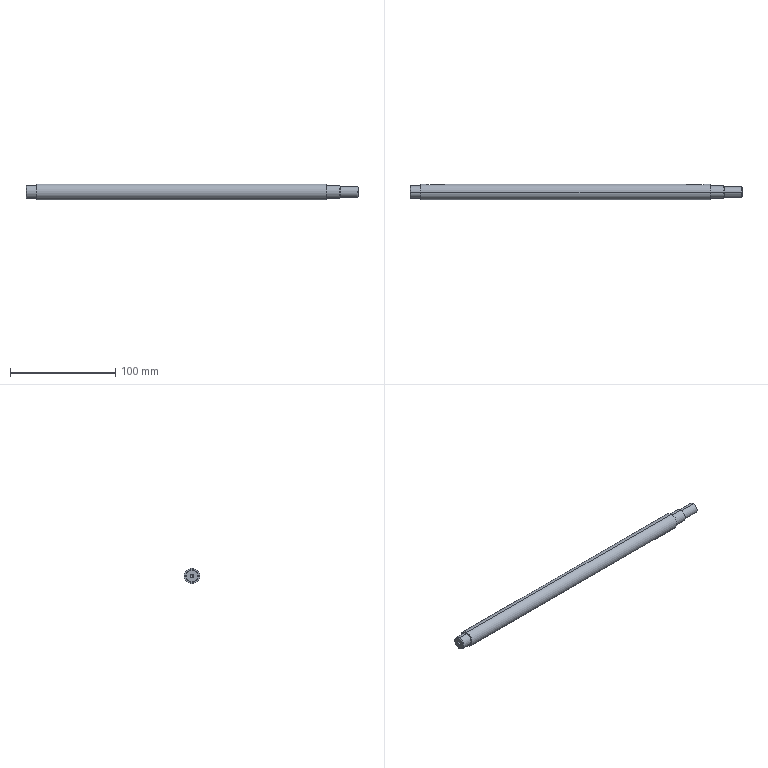Part | STEP file | 11-SS10911 | 1 solid | 42 faces | box 315 x 15 x 15 mm | volume 51716 mm3 | cylinder 18 | plane 14 | cone 10 | commonest cylinder face diameters 3.3 x4 5 x4 12 x4 3 x2 10 x2 15 x2
STEP:
#1=CARTESIAN_POINT('',(304.9,0.,1.65));
#2=VERTEX_POINT('',#1);
#3=CARTESIAN_POINT('',(304.9,0.,-1.65));
#4=VERTEX_POINT('',#3);
#5=CARTESIAN_POINT('',(304.9,0.,0.));
#6=DIRECTION('',(1.,0.,0.));
#7=DIRECTION('',(0.,0.,-1.));
#8=AXIS2_PLACEMENT_3D('',#5,#6,#7);
#9=CIRCLE('',#8,1.65);
#10=EDGE_CURVE('',#2,#4,#9,.T.);
#11=ORIENTED_EDGE('',*,*,#10,.F.);
#12=CARTESIAN_POINT('',(315.,0.,1.65));
#13=VERTEX_POINT('',#12);
#14=CARTESIAN_POINT('',(315.,0.,1.65));
#15=DIRECTION('',(1.,0.,0.));
#16=VECTOR('',#15,1000.);
#17=LINE('',#14,#16);
#18=EDGE_CURVE('',#2,#13,#17,.T.);
#19=ORIENTED_EDGE('',*,*,#18,.T.);
#20=CARTESIAN_POINT('',(315.,0.,-1.65));
#21=VERTEX_POINT('',#20);
#22=CARTESIAN_POINT('',(315.,0.,0.));
#23=DIRECTION('',(1.,0.,0.));
#24=DIRECTION('',(0.,0.,-1.));
#25=AXIS2_PLACEMENT_3D('',#22,#23,#24);
#26=CIRCLE('',#25,1.65);
#27=EDGE_CURVE('',#13,#21,#26,.T.);
#28=ORIENTED_EDGE('',*,*,#27,.T.);
#29=CARTESIAN_POINT('',(315.,0.,-1.65));
#30=DIRECTION('',(1.,0.,0.));
#31=VECTOR('',#30,1000.);
#32=LINE('',#29,#31);
#33=EDGE_CURVE('',#4,#21,#32,.T.);
#34=ORIENTED_EDGE('',*,*,#33,.F.);
#35=EDGE_LOOP('',(#11,#19,#28,#34));
#36=FACE_OUTER_BOUND('',#35,.T.);
#37=CARTESIAN_POINT('',(315.,0.,0.));
#38=DIRECTION('',(1.,0.,0.));
#39=DIRECTION('',(0.,0.,-1.));
#40=AXIS2_PLACEMENT_3D('',#37,#38,#39);
#41=CYLINDRICAL_SURFACE('',#40,1.65);
#42=ADVANCED_FACE('',(#36),#41,.F.);
#43=CARTESIAN_POINT('',(303.909,0.,0.));
#44=VERTEX_POINT('',#43);
#45=CARTESIAN_POINT('',(304.9,0.,-1.65));
#46=DIRECTION('',(0.515,0.,-0.8572));
#47=VECTOR('',#46,1000.);
#48=LINE('',#45,#47);
#49=EDGE_CURVE('',#44,#4,#48,.T.);
#50=ORIENTED_EDGE('',*,*,#49,.F.);
#51=CARTESIAN_POINT('',(304.9,0.,1.65));
#52=DIRECTION('',(0.515,0.,0.8572));
#53=VECTOR('',#52,1000.);
#54=LINE('',#51,#53);
#55=EDGE_CURVE('',#44,#2,#54,.T.);
#56=ORIENTED_EDGE('',*,*,#55,.T.);
#57=ORIENTED_EDGE('',*,*,#10,.T.);
#58=EDGE_LOOP('',(#50,#56,#57));
#59=FACE_OUTER_BOUND('',#58,.T.);
#60=CARTESIAN_POINT('',(304.9,0.,0.));
#61=DIRECTION('',(1.,0.,0.));
#62=DIRECTION('',(0.,0.,-1.));
#63=AXIS2_PLACEMENT_3D('',#60,#61,#62);
#64=CONICAL_SURFACE('',#63,1.65,1.03);
#65=ADVANCED_FACE('',(#59),#64,.F.);
#66=CARTESIAN_POINT('',(10.1,0.,-1.65));
#67=VERTEX_POINT('',#66);
#68=CARTESIAN_POINT('',(10.1,0.,1.65));
#69=VERTEX_POINT('',#68);
#70=CARTESIAN_POINT('',(10.1,0.,0.));
#71=DIRECTION('',(-1.,0.,0.));
#72=DIRECTION('',(0.,0.,1.));
#73=AXIS2_PLACEMENT_3D('',#70,#71,#72);
#74=CIRCLE('',#73,1.65);
#75=EDGE_CURVE('',#67,#69,#74,.T.);
#76=ORIENTED_EDGE('',*,*,#75,.F.);
#77=CARTESIAN_POINT('',(0.,0.,-1.65));
#78=VERTEX_POINT('',#77);
#79=CARTESIAN_POINT('',(0.,0.,-1.65));
#80=DIRECTION('',(-1.,0.,0.));
#81=VECTOR('',#80,1000.);
#82=LINE('',#79,#81);
#83=EDGE_CURVE('',#67,#78,#82,.T.);
#84=ORIENTED_EDGE('',*,*,#83,.T.);
#85=CARTESIAN_POINT('',(0.,0.,1.65));
#86=VERTEX_POINT('',#85);
#87=CARTESIAN_POINT('',(0.,0.,0.));
#88=DIRECTION('',(-1.,0.,0.));
#89=DIRECTION('',(0.,0.,1.));
#90=AXIS2_PLACEMENT_3D('',#87,#88,#89);
#91=CIRCLE('',#90,1.65);
#92=EDGE_CURVE('',#78,#86,#91,.T.);
#93=ORIENTED_EDGE('',*,*,#92,.T.);
#94=CARTESIAN_POINT('',(0.,0.,1.65));
#95=DIRECTION('',(-1.,0.,0.));
#96=VECTOR('',#95,1000.);
#97=LINE('',#94,#96);
#98=EDGE_CURVE('',#69,#86,#97,.T.);
#99=ORIENTED_EDGE('',*,*,#98,.F.);
#100=EDGE_LOOP('',(#76,#84,#93,#99));
#101=FACE_OUTER_BOUND('',#100,.T.);
#102=CARTESIAN_POINT('',(0.,0.,0.));
#103=DIRECTION('',(-1.,0.,0.));
#104=DIRECTION('',(0.,0.,1.));
#105=AXIS2_PLACEMENT_3D('',#102,#103,#104);
#106=CYLINDRICAL_SURFACE('',#105,1.65);
#107=ADVANCED_FACE('',(#101),#106,.F.);
#108=CARTESIAN_POINT('',(11.091,0.,0.));
#109=VERTEX_POINT('',#108);
#110=CARTESIAN_POINT('',(10.1,0.,1.65));
#111=DIRECTION('',(-0.515,0.,0.8572));
#112=VECTOR('',#111,1000.);
#113=LINE('',#110,#112);
#114=EDGE_CURVE('',#109,#69,#113,.T.);
#115=ORIENTED_EDGE('',*,*,#114,.F.);
#116=CARTESIAN_POINT('',(10.1,0.,-1.65));
#117=DIRECTION('',(-0.515,0.,-0.8572));
#118=VECTOR('',#117,1000.);
#119=LINE('',#116,#118);
#120=EDGE_CURVE('',#109,#67,#119,.T.);
#121=ORIENTED_EDGE('',*,*,#120,.T.);
#122=ORIENTED_EDGE('',*,*,#75,.T.);
#123=EDGE_LOOP('',(#115,#121,#122));
#124=FACE_OUTER_BOUND('',#123,.T.);
#125=CARTESIAN_POINT('',(10.1,0.,0.));
#126=DIRECTION('',(-1.,0.,0.));
#127=DIRECTION('',(0.,0.,1.));
#128=AXIS2_PLACEMENT_3D('',#125,#126,#127);
#129=CONICAL_SURFACE('',#128,1.65,1.03);
#130=ADVANCED_FACE('',(#124),#129,.F.);
#131=CARTESIAN_POINT('',(298.,0.,-5.5));
#132=VERTEX_POINT('',#131);
#133=CARTESIAN_POINT('',(298.,0.,5.5));
#134=VERTEX_POINT('',#133);
#135=CARTESIAN_POINT('',(298.,0.,0.));
#136=DIRECTION('',(1.,0.,0.));
#137=DIRECTION('',(0.,0.,1.));
#138=AXIS2_PLACEMENT_3D('',#135,#136,#137);
#139=CIRCLE('',#138,5.5);
#140=EDGE_CURVE('',#132,#134,#139,.T.);
#141=ORIENTED_EDGE('',*,*,#140,.F.);
#142=CARTESIAN_POINT('',(297.5,0.,-6.));
#143=VERTEX_POINT('',#142);
#144=CARTESIAN_POINT('',(297.5,0.,-6.));
#145=DIRECTION('',(-0.7071,0.,-0.7071));
#146=VECTOR('',#145,1000.);
#147=LINE('',#144,#146);
#148=EDGE_CURVE('',#132,#143,#147,.T.);
#149=ORIENTED_EDGE('',*,*,#148,.T.);
#150=CARTESIAN_POINT('',(297.5,0.,6.));
#151=VERTEX_POINT('',#150);
#152=CARTESIAN_POINT('',(297.5,0.,0.));
#153=DIRECTION('',(-1.,0.,0.));
#154=DIRECTION('',(0.,0.,1.));
#155=AXIS2_PLACEMENT_3D('',#152,#153,#154);
#156=CIRCLE('',#155,6.);
#157=EDGE_CURVE('',#151,#143,#156,.T.);
#158=ORIENTED_EDGE('',*,*,#157,.F.);
#159=CARTESIAN_POINT('',(297.5,0.,6.));
#160=DIRECTION('',(-0.7071,0.,0.7071));
#161=VECTOR('',#160,1000.);
#162=LINE('',#159,#161);
#163=EDGE_CURVE('',#134,#151,#162,.T.);
#164=ORIENTED_EDGE('',*,*,#163,.F.);
#165=EDGE_LOOP('',(#141,#149,#158,#164));
#166=FACE_OUTER_BOUND('',#165,.T.);
#167=CARTESIAN_POINT('',(297.5,0.,0.));
#168=DIRECTION('',(-1.,0.,0.));
#169=DIRECTION('',(0.,0.,1.));
#170=AXIS2_PLACEMENT_3D('',#167,#168,#169);
#171=CONICAL_SURFACE('',#170,6.,0.7854);
#172=ADVANCED_FACE('',(#166),#171,.T.);
#173=CARTESIAN_POINT('',(315.,0.,-4.5));
#174=VERTEX_POINT('',#173);
#175=CARTESIAN_POINT('',(315.,0.,4.5));
#176=VERTEX_POINT('',#175);
#177=CARTESIAN_POINT('',(315.,0.,0.));
#178=DIRECTION('',(1.,0.,0.));
#179=DIRECTION('',(0.,0.,1.));
#180=AXIS2_PLACEMENT_3D('',#177,#178,#179);
#181=CIRCLE('',#180,4.5);
#182=EDGE_CURVE('',#174,#176,#181,.T.);
#183=ORIENTED_EDGE('',*,*,#182,.F.);
#184=CARTESIAN_POINT('',(314.5,0.,-5.));
#185=VERTEX_POINT('',#184);
#186=CARTESIAN_POINT('',(314.5,0.,-5.));
#187=DIRECTION('',(-0.7071,0.,-0.7071));
#188=VECTOR('',#187,1000.);
#189=LINE('',#186,#188);
#190=EDGE_CURVE('',#174,#185,#189,.T.);
#191=ORIENTED_EDGE('',*,*,#190,.T.);
#192=CARTESIAN_POINT('',(314.5,0.,5.));
#193=VERTEX_POINT('',#192);
#194=CARTESIAN_POINT('',(314.5,0.,0.));
#195=DIRECTION('',(-1.,0.,0.));
#196=DIRECTION('',(0.,0.,1.));
#197=AXIS2_PLACEMENT_3D('',#194,#195,#196);
#198=CIRCLE('',#197,5.);
#199=EDGE_CURVE('',#193,#185,#198,.T.);
#200=ORIENTED_EDGE('',*,*,#199,.F.);
#201=CARTESIAN_POINT('',(314.5,0.,5.));
#202=DIRECTION('',(-0.7071,0.,0.7071));
#203=VECTOR('',#202,1000.);
#204=LINE('',#201,#203);
#205=EDGE_CURVE('',#176,#193,#204,.T.);
#206=ORIENTED_EDGE('',*,*,#205,.F.);
#207=EDGE_LOOP('',(#183,#191,#200,#206));
#208=FACE_OUTER_BOUND('',#207,.T.);
#209=CARTESIAN_POINT('',(314.5,0.,0.));
#210=DIRECTION('',(-1.,0.,0.));
#211=DIRECTION('',(0.,0.,1.));
#212=AXIS2_PLACEMENT_3D('',#209,#210,#211);
#213=CONICAL_SURFACE('',#212,5.,0.7854);
#214=ADVANCED_FACE('',(#208),#213,.T.);
#215=CARTESIAN_POINT('',(0.,0.,5.5));
#216=VERTEX_POINT('',#215);
#217=CARTESIAN_POINT('',(0.,0.,-5.5));
#218=VERTEX_POINT('',#217);
#219=CARTESIAN_POINT('',(0.,0.,0.));
#220=DIRECTION('',(-1.,0.,0.));
#221=DIRECTION('',(0.,0.,-1.));
#222=AXIS2_PLACEMENT_3D('',#219,#220,#221);
#223=CIRCLE('',#222,5.5);
#224=EDGE_CURVE('',#216,#218,#223,.T.);
#225=ORIENTED_EDGE('',*,*,#224,.F.);
#226=CARTESIAN_POINT('',(0.5,0.,6.));
#227=VERTEX_POINT('',#226);
#228=CARTESIAN_POINT('',(0.,0.,5.5));
#229=DIRECTION('',(0.7071,0.,0.7071));
#230=VECTOR('',#229,1000.);
#231=LINE('',#228,#230);
#232=EDGE_CURVE('',#216,#227,#231,.T.);
#233=ORIENTED_EDGE('',*,*,#232,.T.);
#234=CARTESIAN_POINT('',(0.5,0.,-6.));
#235=VERTEX_POINT('',#234);
#236=CARTESIAN_POINT('',(0.5,0.,0.));
#237=DIRECTION('',(1.,0.,0.));
#238=DIRECTION('',(0.,0.,-1.));
#239=AXIS2_PLACEMENT_3D('',#236,#237,#238);
#240=CIRCLE('',#239,6.);
#241=EDGE_CURVE('',#235,#227,#240,.T.);
#242=ORIENTED_EDGE('',*,*,#241,.F.);
#243=CARTESIAN_POINT('',(0.,0.,-5.5));
#244=DIRECTION('',(0.7071,0.,-0.7071));
#245=VECTOR('',#244,1000.);
#246=LINE('',#243,#245);
#247=EDGE_CURVE('',#218,#235,#246,.T.);
#248=ORIENTED_EDGE('',*,*,#247,.F.);
#249=EDGE_LOOP('',(#225,#233,#242,#248));
#250=FACE_OUTER_BOUND('',#249,.T.);
#251=CARTESIAN_POINT('',(0.,0.,0.));
#252=DIRECTION('',(1.,0.,0.));
#253=DIRECTION('',(0.,0.,-1.));
#254=AXIS2_PLACEMENT_3D('',#251,#252,#253);
#255=CONICAL_SURFACE('',#254,5.5,0.7854);
#256=ADVANCED_FACE('',(#250),#255,.T.);
#257=CARTESIAN_POINT('',(312.,4.77,1.5));
#258=VERTEX_POINT('',#257);
#259=CARTESIAN_POINT('',(300.,4.77,1.5));
#260=VERTEX_POINT('',#259);
#261=CARTESIAN_POINT('',(0.,4.77,1.5));
#262=DIRECTION('',(-1.,0.,0.));
#263=VECTOR('',#262,1000.);
#264=LINE('',#261,#263);
#265=EDGE_CURVE('',#258,#260,#264,.T.);
#266=ORIENTED_EDGE('',*,*,#265,.T.);
#267=CARTESIAN_POINT('',(300.,4.77,-1.5));
#268=VERTEX_POINT('',#267);
#269=CARTESIAN_POINT('',(300.,4.77,1.5));
#270=CARTESIAN_POINT('',(299.9,4.77,1.5));
#271=CARTESIAN_POINT('',(299.802,4.773,1.49));
#272=CARTESIAN_POINT('',(299.61,4.785,1.452));
#273=CARTESIAN_POINT('',(299.514,4.794,1.423));
#274=CARTESIAN_POINT('',(299.333,4.815,1.347));
#275=CARTESIAN_POINT('',(299.247,4.828,1.301));
#276=CARTESIAN_POINT('',(299.085,4.856,1.192));
#277=CARTESIAN_POINT('',(299.008,4.871,1.129));
#278=CARTESIAN_POINT('',(298.802,4.916,0.9233));
#279=CARTESIAN_POINT('',(298.69,4.946,0.7569));
#280=CARTESIAN_POINT('',(298.54,4.988,0.3965));
#281=CARTESIAN_POINT('',(298.5,5.,0.1984));
#282=CARTESIAN_POINT('',(298.5,5.,-0.09698));
#283=CARTESIAN_POINT('',(298.51,4.997,-0.197));
#284=CARTESIAN_POINT('',(298.548,4.986,-0.3898));
#285=CARTESIAN_POINT('',(298.577,4.977,-0.4837));
#286=CARTESIAN_POINT('',(298.69,4.946,-0.7572));
#287=CARTESIAN_POINT('',(298.801,4.916,-0.9219));
#288=CARTESIAN_POINT('',(299.008,4.871,-1.13));
#289=CARTESIAN_POINT('',(299.083,4.856,-1.191));
#290=CARTESIAN_POINT('',(299.245,4.828,-1.3));
#291=CARTESIAN_POINT('',(299.333,4.815,-1.347));
#292=CARTESIAN_POINT('',(299.604,4.783,-1.46));
#293=CARTESIAN_POINT('',(299.801,4.77,-1.5));
#294=CARTESIAN_POINT('',(300.,4.77,-1.5));
#295=B_SPLINE_CURVE_WITH_KNOTS('',3,(#269,#270,#271,#272,#273,#274,#275,#276,#277,#278,#279,#280,#281,#282,#283,#284,#285,#286,#287,#288,#289,#290,#291,#292,#293,#294),.UNSPECIFIED.,.F.,.F.,(4,2,2,2,2,2,2,2,2,2,2,2,4),(0.,0.0002947,0.0005894,0.0008841,0.001179,0.001768,0.002358,0.002652,0.002947,0.003536,0.003831,0.004126,0.004715),.UNSPECIFIED.);
#296=EDGE_CURVE('',#260,#268,#295,.T.);
#297=ORIENTED_EDGE('',*,*,#296,.T.);
#298=CARTESIAN_POINT('',(312.,4.77,-1.5));
#299=VERTEX_POINT('',#298);
#300=CARTESIAN_POINT('',(0.,4.77,-1.5));
#301=DIRECTION('',(1.,0.,0.));
#302=VECTOR('',#301,1000.);
#303=LINE('',#300,#302);
#304=EDGE_CURVE('',#268,#299,#303,.T.);
#305=ORIENTED_EDGE('',*,*,#304,.T.);
#306=CARTESIAN_POINT('',(312.,4.77,-1.5));
#307=CARTESIAN_POINT('',(312.1,4.77,-1.5));
#308=CARTESIAN_POINT('',(312.198,4.773,-1.49));
#309=CARTESIAN_POINT('',(312.39,4.785,-1.452));
#310=CARTESIAN_POINT('',(312.486,4.794,-1.423));
#311=CARTESIAN_POINT('',(312.667,4.815,-1.347));
#312=CARTESIAN_POINT('',(312.753,4.828,-1.301));
#313=CARTESIAN_POINT('',(312.915,4.856,-1.192));
#314=CARTESIAN_POINT('',(312.992,4.871,-1.129));
#315=CARTESIAN_POINT('',(313.198,4.916,-0.9233));
#316=CARTESIAN_POINT('',(313.31,4.946,-0.7569));
#317=CARTESIAN_POINT('',(313.46,4.988,-0.3965));
#318=CARTESIAN_POINT('',(313.5,5.,-0.1984));
#319=CARTESIAN_POINT('',(313.5,5.,0.09698));
#320=CARTESIAN_POINT('',(313.49,4.997,0.197));
#321=CARTESIAN_POINT('',(313.452,4.986,0.3898));
#322=CARTESIAN_POINT('',(313.423,4.977,0.4837));
#323=CARTESIAN_POINT('',(313.31,4.946,0.7572));
#324=CARTESIAN_POINT('',(313.199,4.916,0.9219));
#325=CARTESIAN_POINT('',(312.992,4.871,1.13));
#326=CARTESIAN_POINT('',(312.917,4.856,1.191));
#327=CARTESIAN_POINT('',(312.755,4.828,1.3));
#328=CARTESIAN_POINT('',(312.667,4.815,1.347));
#329=CARTESIAN_POINT('',(312.396,4.783,1.46));
#330=CARTESIAN_POINT('',(312.199,4.77,1.5));
#331=CARTESIAN_POINT('',(312.,4.77,1.5));
#332=B_SPLINE_CURVE_WITH_KNOTS('',3,(#306,#307,#308,#309,#310,#311,#312,#313,#314,#315,#316,#317,#318,#319,#320,#321,#322,#323,#324,#325,#326,#327,#328,#329,#330,#331),.UNSPECIFIED.,.F.,.F.,(4,2,2,2,2,2,2,2,2,2,2,2,4),(0.,0.0002947,0.0005894,0.0008841,0.001179,0.001768,0.002358,0.002652,0.002947,0.003536,0.003831,0.004126,0.004715),.UNSPECIFIED.);
#333=EDGE_CURVE('',#299,#258,#332,.T.);
#334=ORIENTED_EDGE('',*,*,#333,.T.);
#335=EDGE_LOOP('',(#266,#297,#305,#334));
#336=FACE_BOUND('',#335,.T.);
#337=ORIENTED_EDGE('',*,*,#199,.T.);
#338=CARTESIAN_POINT('',(298.,0.,-5.));
#339=VERTEX_POINT('',#338);
#340=CARTESIAN_POINT('',(0.,0.,-5.));
#341=DIRECTION('',(-1.,0.,0.));
#342=VECTOR('',#341,1000.);
#343=LINE('',#340,#342);
#344=EDGE_CURVE('',#185,#339,#343,.T.);
#345=ORIENTED_EDGE('',*,*,#344,.T.);
#346=CARTESIAN_POINT('',(298.,0.,5.));
#347=VERTEX_POINT('',#346);
#348=CARTESIAN_POINT('',(298.,0.,0.));
#349=DIRECTION('',(-1.,0.,0.));
#350=DIRECTION('',(0.,0.,1.));
#351=AXIS2_PLACEMENT_3D('',#348,#349,#350);
#352=CIRCLE('',#351,5.);
#353=EDGE_CURVE('',#347,#339,#352,.T.);
#354=ORIENTED_EDGE('',*,*,#353,.F.);
#355=CARTESIAN_POINT('',(0.,0.,5.));
#356=DIRECTION('',(-1.,0.,0.));
#357=VECTOR('',#356,1000.);
#358=LINE('',#355,#357);
#359=EDGE_CURVE('',#193,#347,#358,.T.);
#360=ORIENTED_EDGE('',*,*,#359,.F.);
#361=EDGE_LOOP('',(#337,#345,#354,#360));
#362=FACE_OUTER_BOUND('',#361,.T.);
#363=CARTESIAN_POINT('',(0.,0.,0.));
#364=DIRECTION('',(-1.,0.,0.));
#365=DIRECTION('',(0.,0.,1.));
#366=AXIS2_PLACEMENT_3D('',#363,#364,#365);
#367=CYLINDRICAL_SURFACE('',#366,5.);
#368=ADVANCED_FACE('',(#336,#362),#367,.T.);
#369=ORIENTED_EDGE('',*,*,#157,.T.);
#370=CARTESIAN_POINT('',(285.,0.,-6.));
#371=VERTEX_POINT('',#370);
#372=CARTESIAN_POINT('',(0.,0.,-6.));
#373=DIRECTION('',(-1.,0.,0.));
#374=VECTOR('',#373,1000.);
#375=LINE('',#372,#374);
#376=EDGE_CURVE('',#143,#371,#375,.T.);
#377=ORIENTED_EDGE('',*,*,#376,.T.);
#378=CARTESIAN_POINT('',(285.,0.,6.));
#379=VERTEX_POINT('',#378);
#380=CARTESIAN_POINT('',(285.,0.,0.));
#381=DIRECTION('',(-1.,0.,0.));
#382=DIRECTION('',(0.,0.,1.));
#383=AXIS2_PLACEMENT_3D('',#380,#381,#382);
#384=CIRCLE('',#383,6.);
#385=EDGE_CURVE('',#379,#371,#384,.T.);
#386=ORIENTED_EDGE('',*,*,#385,.F.);
#387=CARTESIAN_POINT('',(0.,0.,6.));
#388=DIRECTION('',(-1.,0.,0.));
#389=VECTOR('',#388,1000.);
#390=LINE('',#387,#389);
#391=EDGE_CURVE('',#151,#379,#390,.T.);
#392=ORIENTED_EDGE('',*,*,#391,.F.);
#393=EDGE_LOOP('',(#369,#377,#386,#392));
#394=FACE_OUTER_BOUND('',#393,.T.);
#395=CARTESIAN_POINT('',(0.,0.,0.));
#396=DIRECTION('',(-1.,0.,0.));
#397=DIRECTION('',(0.,0.,1.));
#398=AXIS2_PLACEMENT_3D('',#395,#396,#397);
#399=CYLINDRICAL_SURFACE('',#398,6.);
#400=ADVANCED_FACE('',(#394),#399,.T.);
#401=CARTESIAN_POINT('',(278.,7.071,2.5));
#402=VERTEX_POINT('',#401);
#403=CARTESIAN_POINT('',(263.,7.071,2.5));
#404=VERTEX_POINT('',#403);
#405=CARTESIAN_POINT('',(0.,7.071,2.5));
#406=DIRECTION('',(-1.,0.,0.));
#407=VECTOR('',#406,1000.);
#408=LINE('',#405,#407);
#409=EDGE_CURVE('',#402,#404,#408,.T.);
#410=ORIENTED_EDGE('',*,*,#409,.T.);
#411=CARTESIAN_POINT('',(263.,7.071,-2.5));
#412=VERTEX_POINT('',#411);
#413=CARTESIAN_POINT('',(263.,7.071,2.5));
#414=CARTESIAN_POINT('',(262.834,7.071,2.5));
#415=CARTESIAN_POINT('',(262.67,7.077,2.484));
#416=CARTESIAN_POINT('',(262.349,7.099,2.419));
#417=CARTESIAN_POINT('',(262.19,7.116,2.371));
#418=CARTESIAN_POINT('',(261.888,7.156,2.245));
#419=CARTESIAN_POINT('',(261.745,7.18,2.168));
#420=CARTESIAN_POINT('',(261.474,7.233,1.987));
#421=CARTESIAN_POINT('',(261.347,7.261,1.882));
#422=CARTESIAN_POINT('',(261.004,7.344,1.539));
#423=CARTESIAN_POINT('',(260.818,7.399,1.262));
#424=CARTESIAN_POINT('',(260.63,7.457,0.812));
#425=CARTESIAN_POINT('',(260.581,7.473,0.6532));
#426=CARTESIAN_POINT('',(260.516,7.494,0.33));
#427=CARTESIAN_POINT('',(260.5,7.5,0.167));
#428=CARTESIAN_POINT('',(260.5,7.5,-0.1617));
#429=CARTESIAN_POINT('',(260.516,7.495,-0.3287));
#430=CARTESIAN_POINT('',(260.58,7.473,-0.6503));
#431=CARTESIAN_POINT('',(260.628,7.458,-0.8068));
#432=CARTESIAN_POINT('',(260.754,7.419,-1.111));
#433=CARTESIAN_POINT('',(260.832,7.395,-1.255));
#434=CARTESIAN_POINT('',(261.012,7.345,-1.525));
#435=CARTESIAN_POINT('',(261.117,7.317,-1.652));
#436=CARTESIAN_POINT('',(261.347,7.261,-1.882));
#437=CARTESIAN_POINT('',(261.472,7.233,-1.985));
#438=CARTESIAN_POINT('',(261.741,7.181,-2.166));
#439=CARTESIAN_POINT('',(261.887,7.156,-2.245));
#440=CARTESIAN_POINT('',(262.188,7.116,-2.37));
#441=CARTESIAN_POINT('',(262.344,7.1,-2.418));
#442=CARTESIAN_POINT('',(262.667,7.077,-2.483));
#443=CARTESIAN_POINT('',(262.834,7.071,-2.5));
#444=CARTESIAN_POINT('',(263.,7.071,-2.5));
#445=B_SPLINE_CURVE_WITH_KNOTS('',3,(#413,#414,#415,#416,#417,#418,#419,#420,#421,#422,#423,#424,#425,#426,#427,#428,#429,#430,#431,#432,#433,#434,#435,#436,#437,#438,#439,#440,#441,#442,#443,#444),.UNSPECIFIED.,.F.,.F.,(4,2,2,2,2,2,2,2,2,2,2,2,2,2,2,4),(0.,0.0004919,0.0009837,0.001476,0.001967,0.002951,0.003443,0.003935,0.004427,0.004919,0.00541,0.005902,0.006394,0.006886,0.007378,0.00787),.UNSPECIFIED.);
#446=EDGE_CURVE('',#404,#412,#445,.T.);
#447=ORIENTED_EDGE('',*,*,#446,.T.);
#448=CARTESIAN_POINT('',(278.,7.071,-2.5));
#449=VERTEX_POINT('',#448);
#450=CARTESIAN_POINT('',(0.,7.071,-2.5));
#451=DIRECTION('',(1.,0.,0.));
#452=VECTOR('',#451,1000.);
#453=LINE('',#450,#452);
#454=EDGE_CURVE('',#412,#449,#453,.T.);
#455=ORIENTED_EDGE('',*,*,#454,.T.);
#456=CARTESIAN_POINT('',(278.,7.071,-2.5));
#457=CARTESIAN_POINT('',(278.164,7.071,-2.5));
#458=CARTESIAN_POINT('',(278.329,7.077,-2.484));
#459=CARTESIAN_POINT('',(278.653,7.099,-2.419));
#460=CARTESIAN_POINT('',(278.81,7.116,-2.371));
#461=CARTESIAN_POINT('',(279.111,7.156,-2.245));
#462=CARTESIAN_POINT('',(279.257,7.181,-2.167));
#463=CARTESIAN_POINT('',(279.527,7.233,-1.986));
#464=CARTESIAN_POINT('',(279.652,7.261,-1.883));
#465=CARTESIAN_POINT('',(279.999,7.345,-1.537));
#466=CARTESIAN_POINT('',(280.182,7.399,-1.264));
#467=CARTESIAN_POINT('',(280.371,7.458,-0.8084));
#468=CARTESIAN_POINT('',(280.419,7.473,-0.6521));
#469=CARTESIAN_POINT('',(280.483,7.494,-0.3312));
#470=CARTESIAN_POINT('',(280.5,7.5,-0.1644));
#471=CARTESIAN_POINT('',(280.5,7.5,0.1651));
#472=CARTESIAN_POINT('',(280.484,7.495,0.3282));
#473=CARTESIAN_POINT('',(280.419,7.473,0.6514));
#474=CARTESIAN_POINT('',(280.371,7.458,0.8105));
#475=CARTESIAN_POINT('',(280.183,7.399,1.262));
#476=CARTESIAN_POINT('',(279.997,7.344,1.539));
#477=CARTESIAN_POINT('',(279.653,7.261,1.883));
#478=CARTESIAN_POINT('',(279.525,7.233,1.987));
#479=CARTESIAN_POINT('',(279.255,7.18,2.168));
#480=CARTESIAN_POINT('',(279.112,7.156,2.245));
#481=CARTESIAN_POINT('',(278.81,7.116,2.371));
#482=CARTESIAN_POINT('',(278.651,7.099,2.419));
#483=CARTESIAN_POINT('',(278.33,7.077,2.484));
#484=CARTESIAN_POINT('',(278.166,7.071,2.5));
#485=CARTESIAN_POINT('',(278.,7.071,2.5));
#486=B_SPLINE_CURVE_WITH_KNOTS('',3,(#456,#457,#458,#459,#460,#461,#462,#463,#464,#465,#466,#467,#468,#469,#470,#471,#472,#473,#474,#475,#476,#477,#478,#479,#480,#481,#482,#483,#484,#485),.UNSPECIFIED.,.F.,.F.,(4,2,2,2,2,2,2,2,2,2,2,2,2,2,4),(0.007873,0.008365,0.008857,0.009348,0.00984,0.01082,0.01132,0.01181,0.0123,0.01279,0.01378,0.01427,0.01476,0.01525,0.01574),.UNSPECIFIED.);
#487=EDGE_CURVE('',#449,#402,#486,.T.);
#488=ORIENTED_EDGE('',*,*,#487,.T.);
#489=EDGE_LOOP('',(#410,#447,#455,#488));
#490=FACE_BOUND('',#489,.T.);
#491=CARTESIAN_POINT('',(17.,7.071,-2.5));
#492=VERTEX_POINT('',#491);
#493=CARTESIAN_POINT('',(32.,7.071,-2.5));
#494=VERTEX_POINT('',#493);
#495=CARTESIAN_POINT('',(0.,7.071,-2.5));
#496=DIRECTION('',(1.,0.,0.));
#497=VECTOR('',#496,1000.);
#498=LINE('',#495,#497);
#499=EDGE_CURVE('',#492,#494,#498,.T.);
#500=ORIENTED_EDGE('',*,*,#499,.T.);
#501=CARTESIAN_POINT('',(32.,7.071,2.5));
#502=VERTEX_POINT('',#501);
#503=CARTESIAN_POINT('',(32.,7.071,-2.5));
#504=CARTESIAN_POINT('',(32.164,7.071,-2.5));
#505=CARTESIAN_POINT('',(32.329,7.077,-2.484));
#506=CARTESIAN_POINT('',(32.653,7.099,-2.419));
#507=CARTESIAN_POINT('',(32.81,7.116,-2.371));
#508=CARTESIAN_POINT('',(33.111,7.156,-2.245));
#509=CARTESIAN_POINT('',(33.257,7.181,-2.167));
#510=CARTESIAN_POINT('',(33.527,7.233,-1.986));
#511=CARTESIAN_POINT('',(33.652,7.261,-1.883));
#512=CARTESIAN_POINT('',(33.999,7.345,-1.537));
#513=CARTESIAN_POINT('',(34.182,7.399,-1.264));
#514=CARTESIAN_POINT('',(34.371,7.458,-0.8084));
#515=CARTESIAN_POINT('',(34.419,7.473,-0.6521));
#516=CARTESIAN_POINT('',(34.483,7.494,-0.3312));
#517=CARTESIAN_POINT('',(34.5,7.5,-0.1644));
#518=CARTESIAN_POINT('',(34.5,7.5,0.1651));
#519=CARTESIAN_POINT('',(34.484,7.495,0.3282));
#520=CARTESIAN_POINT('',(34.419,7.473,0.6514));
#521=CARTESIAN_POINT('',(34.371,7.458,0.8105));
#522=CARTESIAN_POINT('',(34.183,7.399,1.262));
#523=CARTESIAN_POINT('',(33.997,7.344,1.539));
#524=CARTESIAN_POINT('',(33.653,7.261,1.883));
#525=CARTESIAN_POINT('',(33.525,7.233,1.987));
#526=CARTESIAN_POINT('',(33.255,7.18,2.168));
#527=CARTESIAN_POINT('',(33.112,7.156,2.245));
#528=CARTESIAN_POINT('',(32.81,7.116,2.371));
#529=CARTESIAN_POINT('',(32.651,7.099,2.419));
#530=CARTESIAN_POINT('',(32.33,7.077,2.484));
#531=CARTESIAN_POINT('',(32.166,7.071,2.5));
#532=CARTESIAN_POINT('',(32.,7.071,2.5));
#533=B_SPLINE_CURVE_WITH_KNOTS('',3,(#503,#504,#505,#506,#507,#508,#509,#510,#511,#512,#513,#514,#515,#516,#517,#518,#519,#520,#521,#522,#523,#524,#525,#526,#527,#528,#529,#530,#531,#532),.UNSPECIFIED.,.F.,.F.,(4,2,2,2,2,2,2,2,2,2,2,2,2,2,4),(0.007873,0.008365,0.008857,0.009348,0.00984,0.01082,0.01132,0.01181,0.0123,0.01279,0.01378,0.01427,0.01476,0.01525,0.01574),.UNSPECIFIED.);
#534=EDGE_CURVE('',#494,#502,#533,.T.);
#535=ORIENTED_EDGE('',*,*,#534,.T.);
#536=CARTESIAN_POINT('',(17.,7.071,2.5));
#537=VERTEX_POINT('',#536);
#538=CARTESIAN_POINT('',(0.,7.071,2.5));
#539=DIRECTION('',(-1.,0.,0.));
#540=VECTOR('',#539,1000.);
#541=LINE('',#538,#540);
#542=EDGE_CURVE('',#502,#537,#541,.T.);
#543=ORIENTED_EDGE('',*,*,#542,.T.);
#544=CARTESIAN_POINT('',(17.,7.071,2.5));
#545=CARTESIAN_POINT('',(16.834,7.071,2.5));
#546=CARTESIAN_POINT('',(16.67,7.077,2.484));
#547=CARTESIAN_POINT('',(16.349,7.099,2.419));
#548=CARTESIAN_POINT('',(16.19,7.116,2.371));
#549=CARTESIAN_POINT('',(15.888,7.156,2.245));
#550=CARTESIAN_POINT('',(15.745,7.18,2.168));
#551=CARTESIAN_POINT('',(15.474,7.233,1.987));
#552=CARTESIAN_POINT('',(15.347,7.261,1.882));
#553=CARTESIAN_POINT('',(15.004,7.344,1.539));
#554=CARTESIAN_POINT('',(14.818,7.399,1.262));
#555=CARTESIAN_POINT('',(14.63,7.457,0.812));
#556=CARTESIAN_POINT('',(14.581,7.473,0.6532));
#557=CARTESIAN_POINT('',(14.516,7.494,0.33));
#558=CARTESIAN_POINT('',(14.5,7.5,0.167));
#559=CARTESIAN_POINT('',(14.5,7.5,-0.1617));
#560=CARTESIAN_POINT('',(14.516,7.495,-0.3287));
#561=CARTESIAN_POINT('',(14.58,7.473,-0.6503));
#562=CARTESIAN_POINT('',(14.628,7.458,-0.8068));
#563=CARTESIAN_POINT('',(14.754,7.419,-1.111));
#564=CARTESIAN_POINT('',(14.832,7.395,-1.255));
#565=CARTESIAN_POINT('',(15.012,7.345,-1.525));
#566=CARTESIAN_POINT('',(15.117,7.317,-1.652));
#567=CARTESIAN_POINT('',(15.347,7.261,-1.882));
#568=CARTESIAN_POINT('',(15.472,7.233,-1.985));
#569=CARTESIAN_POINT('',(15.741,7.181,-2.166));
#570=CARTESIAN_POINT('',(15.887,7.156,-2.245));
#571=CARTESIAN_POINT('',(16.188,7.116,-2.37));
#572=CARTESIAN_POINT('',(16.344,7.1,-2.418));
#573=CARTESIAN_POINT('',(16.667,7.077,-2.483));
#574=CARTESIAN_POINT('',(16.834,7.071,-2.5));
#575=CARTESIAN_POINT('',(17.,7.071,-2.5));
#576=B_SPLINE_CURVE_WITH_KNOTS('',3,(#544,#545,#546,#547,#548,#549,#550,#551,#552,#553,#554,#555,#556,#557,#558,#559,#560,#561,#562,#563,#564,#565,#566,#567,#568,#569,#570,#571,#572,#573,#574,#575),.UNSPECIFIED.,.F.,.F.,(4,2,2,2,2,2,2,2,2,2,2,2,2,2,2,4),(0.,0.0004919,0.0009837,0.001476,0.001967,0.002951,0.003443,0.003935,0.004427,0.004919,0.00541,0.005902,0.006394,0.006886,0.007378,0.00787),.UNSPECIFIED.);
#577=EDGE_CURVE('',#537,#492,#576,.T.);
#578=ORIENTED_EDGE('',*,*,#577,.T.);
#579=EDGE_LOOP('',(#500,#535,#543,#578));
#580=FACE_BOUND('',#579,.T.);
#581=CARTESIAN_POINT('',(285.,0.,7.5));
#582=VERTEX_POINT('',#581);
#583=CARTESIAN_POINT('',(285.,0.,-7.5));
#584=VERTEX_POINT('',#583);
#585=CARTESIAN_POINT('',(285.,0.,0.));
#586=DIRECTION('',(-1.,0.,0.));
#587=DIRECTION('',(0.,0.,1.));
#588=AXIS2_PLACEMENT_3D('',#585,#586,#587);
#589=CIRCLE('',#588,7.5);
#590=EDGE_CURVE('',#582,#584,#589,.T.);
#591=ORIENTED_EDGE('',*,*,#590,.T.);
#592=CARTESIAN_POINT('',(10.,0.,-7.5));
#593=VERTEX_POINT('',#592);
#594=CARTESIAN_POINT('',(0.,0.,-7.5));
#595=DIRECTION('',(-1.,0.,0.));
#596=VECTOR('',#595,1000.);
#597=LINE('',#594,#596);
#598=EDGE_CURVE('',#584,#593,#597,.T.);
#599=ORIENTED_EDGE('',*,*,#598,.T.);
#600=CARTESIAN_POINT('',(10.,0.,7.5));
#601=VERTEX_POINT('',#600);
#602=CARTESIAN_POINT('',(10.,0.,0.));
#603=DIRECTION('',(-1.,0.,0.));
#604=DIRECTION('',(0.,0.,1.));
#605=AXIS2_PLACEMENT_3D('',#602,#603,#604);
#606=CIRCLE('',#605,7.5);
#607=EDGE_CURVE('',#601,#593,#606,.T.);
#608=ORIENTED_EDGE('',*,*,#607,.F.);
#609=CARTESIAN_POINT('',(0.,0.,7.5));
#610=DIRECTION('',(-1.,0.,0.));
#611=VECTOR('',#610,1000.);
#612=LINE('',#609,#611);
#613=EDGE_CURVE('',#582,#601,#612,.T.);
#614=ORIENTED_EDGE('',*,*,#613,.F.);
#615=EDGE_LOOP('',(#591,#599,#608,#614));
#616=FACE_OUTER_BOUND('',#615,.T.);
#617=CARTESIAN_POINT('',(0.,0.,0.));
#618=DIRECTION('',(-1.,0.,0.));
#619=DIRECTION('',(0.,0.,1.));
#620=AXIS2_PLACEMENT_3D('',#617,#618,#619);
#621=CYLINDRICAL_SURFACE('',#620,7.5);
#622=ADVANCED_FACE('',(#490,#580,#616),#621,.T.);
#623=CARTESIAN_POINT('',(10.,0.,6.));
#624=VERTEX_POINT('',#623);
#625=CARTESIAN_POINT('',(10.,0.,-6.));
#626=VERTEX_POINT('',#625);
#627=CARTESIAN_POINT('',(10.,0.,0.));
#628=DIRECTION('',(-1.,0.,0.));
#629=DIRECTION('',(0.,0.,1.));
#630=AXIS2_PLACEMENT_3D('',#627,#628,#629);
#631=CIRCLE('',#630,6.);
#632=EDGE_CURVE('',#624,#626,#631,.T.);
#633=ORIENTED_EDGE('',*,*,#632,.T.);
#634=CARTESIAN_POINT('',(0.,0.,-6.));
#635=DIRECTION('',(-1.,0.,0.));
#636=VECTOR('',#635,1000.);
#637=LINE('',#634,#636);
#638=EDGE_CURVE('',#626,#235,#637,.T.);
#639=ORIENTED_EDGE('',*,*,#638,.T.);
#640=ORIENTED_EDGE('',*,*,#241,.T.);
#641=CARTESIAN_POINT('',(0.,0.,6.));
#642=DIRECTION('',(-1.,0.,0.));
#643=VECTOR('',#642,1000.);
#644=LINE('',#641,#643);
#645=EDGE_CURVE('',#624,#227,#644,.T.);
#646=ORIENTED_EDGE('',*,*,#645,.F.);
#647=EDGE_LOOP('',(#633,#639,#640,#646));
#648=FACE_OUTER_BOUND('',#647,.T.);
#649=CARTESIAN_POINT('',(0.,0.,0.));
#650=DIRECTION('',(-1.,0.,0.));
#651=DIRECTION('',(0.,0.,1.));
#652=AXIS2_PLACEMENT_3D('',#649,#650,#651);
#653=CYLINDRICAL_SURFACE('',#652,6.);
#654=ADVANCED_FACE('',(#648),#653,.T.);
#655=CARTESIAN_POINT('',(0.,0.,0.));
#656=DIRECTION('',(-1.,0.,0.));
#657=DIRECTION('',(0.,0.,1.));
#658=AXIS2_PLACEMENT_3D('',#655,#656,#657);
#659=CIRCLE('',#658,1.65);
#660=EDGE_CURVE('',#86,#78,#659,.T.);
#661=ORIENTED_EDGE('',*,*,#660,.F.);
#662=ORIENTED_EDGE('',*,*,#92,.F.);
#663=EDGE_LOOP('',(#661,#662));
#664=FACE_BOUND('',#663,.T.);
#665=CARTESIAN_POINT('',(0.,0.,0.));
#666=DIRECTION('',(-1.,0.,0.));
#667=DIRECTION('',(0.,0.,-1.));
#668=AXIS2_PLACEMENT_3D('',#665,#666,#667);
#669=CIRCLE('',#668,5.5);
#670=EDGE_CURVE('',#218,#216,#669,.T.);
#671=ORIENTED_EDGE('',*,*,#670,.T.);
#672=ORIENTED_EDGE('',*,*,#224,.T.);
#673=EDGE_LOOP('',(#671,#672));
#674=FACE_OUTER_BOUND('',#673,.T.);
#675=CARTESIAN_POINT('',(0.,0.,0.));
#676=DIRECTION('',(1.,0.,0.));
#677=DIRECTION('',(0.,0.,-1.));
#678=AXIS2_PLACEMENT_3D('',#675,#676,#677);
#679=PLANE('',#678);
#680=ADVANCED_FACE('',(#664,#674),#679,.F.);
#681=ORIENTED_EDGE('',*,*,#638,.F.);
#682=CARTESIAN_POINT('',(10.,0.,0.));
#683=DIRECTION('',(-1.,0.,0.));
#684=DIRECTION('',(0.,0.,1.));
#685=AXIS2_PLACEMENT_3D('',#682,#683,#684);
#686=CIRCLE('',#685,6.);
#687=EDGE_CURVE('',#626,#624,#686,.T.);
#688=ORIENTED_EDGE('',*,*,#687,.T.);
#689=ORIENTED_EDGE('',*,*,#645,.T.);
#690=CARTESIAN_POINT('',(0.5,0.,0.));
#691=DIRECTION('',(1.,0.,0.));
#692=DIRECTION('',(0.,0.,-1.));
#693=AXIS2_PLACEMENT_3D('',#690,#691,#692);
#694=CIRCLE('',#693,6.);
#695=EDGE_CURVE('',#227,#235,#694,.T.);
#696=ORIENTED_EDGE('',*,*,#695,.T.);
#697=EDGE_LOOP('',(#681,#688,#689,#696));
#698=FACE_OUTER_BOUND('',#697,.T.);
#699=CARTESIAN_POINT('',(0.,0.,0.));
#700=DIRECTION('',(-1.,0.,0.));
#701=DIRECTION('',(0.,0.,1.));
#702=AXIS2_PLACEMENT_3D('',#699,#700,#701);
#703=CYLINDRICAL_SURFACE('',#702,6.);
#704=ADVANCED_FACE('',(#698),#703,.T.);
#705=ORIENTED_EDGE('',*,*,#632,.F.);
#706=ORIENTED_EDGE('',*,*,#687,.F.);
#707=EDGE_LOOP('',(#705,#706));
#708=FACE_BOUND('',#707,.T.);
#709=ORIENTED_EDGE('',*,*,#607,.T.);
#710=CARTESIAN_POINT('',(10.,0.,0.));
#711=DIRECTION('',(-1.,0.,0.));
#712=DIRECTION('',(0.,0.,1.));
#713=AXIS2_PLACEMENT_3D('',#710,#711,#712);
#714=CIRCLE('',#713,7.5);
#715=EDGE_CURVE('',#593,#601,#714,.T.);
#716=ORIENTED_EDGE('',*,*,#715,.T.);
#717=EDGE_LOOP('',(#709,#716));
#718=FACE_OUTER_BOUND('',#717,.T.);
#719=CARTESIAN_POINT('',(10.,6.,0.));
#720=DIRECTION('',(1.,0.,0.));
#721=DIRECTION('',(0.,0.,-1.));
#722=AXIS2_PLACEMENT_3D('',#719,#720,#721);
#723=PLANE('',#722);
#724=ADVANCED_FACE('',(#708,#718),#723,.F.);
#725=ORIENTED_EDGE('',*,*,#598,.F.);
#726=CARTESIAN_POINT('',(285.,0.,0.));
#727=DIRECTION('',(-1.,0.,0.));
#728=DIRECTION('',(0.,0.,1.));
#729=AXIS2_PLACEMENT_3D('',#726,#727,#728);
#730=CIRCLE('',#729,7.5);
#731=EDGE_CURVE('',#584,#582,#730,.T.);
#732=ORIENTED_EDGE('',*,*,#731,.T.);
#733=ORIENTED_EDGE('',*,*,#613,.T.);
#734=ORIENTED_EDGE('',*,*,#715,.F.);
#735=EDGE_LOOP('',(#725,#732,#733,#734));
#736=FACE_OUTER_BOUND('',#735,.T.);
#737=CARTESIAN_POINT('',(0.,0.,0.));
#738=DIRECTION('',(-1.,0.,0.));
#739=DIRECTION('',(0.,0.,1.));
#740=AXIS2_PLACEMENT_3D('',#737,#738,#739);
#741=CYLINDRICAL_SURFACE('',#740,7.5);
#742=ADVANCED_FACE('',(#736),#741,.T.);
#743=ORIENTED_EDGE('',*,*,#590,.F.);
#744=ORIENTED_EDGE('',*,*,#731,.F.);
#745=EDGE_LOOP('',(#743,#744));
#746=FACE_OUTER_BOUND('',#745,.T.);
#747=ORIENTED_EDGE('',*,*,#385,.T.);
#748=CARTESIAN_POINT('',(285.,0.,0.));
#749=DIRECTION('',(-1.,0.,0.));
#750=DIRECTION('',(0.,0.,1.));
#751=AXIS2_PLACEMENT_3D('',#748,#749,#750);
#752=CIRCLE('',#751,6.);
#753=EDGE_CURVE('',#371,#379,#752,.T.);
#754=ORIENTED_EDGE('',*,*,#753,.T.);
#755=EDGE_LOOP('',(#747,#754));
#756=FACE_BOUND('',#755,.T.);
#757=CARTESIAN_POINT('',(285.,7.5,0.));
#758=DIRECTION('',(-1.,0.,0.));
#759=DIRECTION('',(0.,0.,1.));
#760=AXIS2_PLACEMENT_3D('',#757,#758,#759);
#761=PLANE('',#760);
#762=ADVANCED_FACE('',(#746,#756),#761,.F.);
#763=ORIENTED_EDGE('',*,*,#376,.F.);
#764=CARTESIAN_POINT('',(297.5,0.,0.));
#765=DIRECTION('',(-1.,0.,0.));
#766=DIRECTION('',(0.,0.,1.));
#767=AXIS2_PLACEMENT_3D('',#764,#765,#766);
#768=CIRCLE('',#767,6.);
#769=EDGE_CURVE('',#143,#151,#768,.T.);
#770=ORIENTED_EDGE('',*,*,#769,.T.);
#771=ORIENTED_EDGE('',*,*,#391,.T.);
#772=ORIENTED_EDGE('',*,*,#753,.F.);
#773=EDGE_LOOP('',(#763,#770,#771,#772));
#774=FACE_OUTER_BOUND('',#773,.T.);
#775=CARTESIAN_POINT('',(0.,0.,0.));
#776=DIRECTION('',(-1.,0.,0.));
#777=DIRECTION('',(0.,0.,1.));
#778=AXIS2_PLACEMENT_3D('',#775,#776,#777);
#779=CYLINDRICAL_SURFACE('',#778,6.);
#780=ADVANCED_FACE('',(#774),#779,.T.);
#781=CARTESIAN_POINT('',(298.,0.,0.));
#782=DIRECTION('',(1.,0.,0.));
#783=DIRECTION('',(0.,0.,1.));
#784=AXIS2_PLACEMENT_3D('',#781,#782,#783);
#785=CIRCLE('',#784,5.5);
#786=EDGE_CURVE('',#134,#132,#785,.T.);
#787=ORIENTED_EDGE('',*,*,#786,.T.);
#788=ORIENTED_EDGE('',*,*,#140,.T.);
#789=EDGE_LOOP('',(#787,#788));
#790=FACE_OUTER_BOUND('',#789,.T.);
#791=ORIENTED_EDGE('',*,*,#353,.T.);
#792=CARTESIAN_POINT('',(298.,0.,0.));
#793=DIRECTION('',(-1.,0.,0.));
#794=DIRECTION('',(0.,0.,1.));
#795=AXIS2_PLACEMENT_3D('',#792,#793,#794);
#796=CIRCLE('',#795,5.);
#797=EDGE_CURVE('',#339,#347,#796,.T.);
#798=ORIENTED_EDGE('',*,*,#797,.T.);
#799=EDGE_LOOP('',(#791,#798));
#800=FACE_BOUND('',#799,.T.);
#801=CARTESIAN_POINT('',(298.,6.,0.));
#802=DIRECTION('',(-1.,0.,0.));
#803=DIRECTION('',(0.,0.,1.));
#804=AXIS2_PLACEMENT_3D('',#801,#802,#803);
#805=PLANE('',#804);
#806=ADVANCED_FACE('',(#790,#800),#805,.F.);
#807=ORIENTED_EDGE('',*,*,#344,.F.);
#808=CARTESIAN_POINT('',(314.5,0.,0.));
#809=DIRECTION('',(-1.,0.,0.));
#810=DIRECTION('',(0.,0.,1.));
#811=AXIS2_PLACEMENT_3D('',#808,#809,#810);
#812=CIRCLE('',#811,5.);
#813=EDGE_CURVE('',#185,#193,#812,.T.);
#814=ORIENTED_EDGE('',*,*,#813,.T.);
#815=ORIENTED_EDGE('',*,*,#359,.T.);
#816=ORIENTED_EDGE('',*,*,#797,.F.);
#817=EDGE_LOOP('',(#807,#814,#815,#816));
#818=FACE_OUTER_BOUND('',#817,.T.);
#819=CARTESIAN_POINT('',(0.,0.,0.));
#820=DIRECTION('',(-1.,0.,0.));
#821=DIRECTION('',(0.,0.,1.));
#822=AXIS2_PLACEMENT_3D('',#819,#820,#821);
#823=CYLINDRICAL_SURFACE('',#822,5.);
#824=ADVANCED_FACE('',(#818),#823,.T.);
#825=CARTESIAN_POINT('',(315.,0.,0.));
#826=DIRECTION('',(1.,0.,0.));
#827=DIRECTION('',(0.,0.,-1.));
#828=AXIS2_PLACEMENT_3D('',#825,#826,#827);
#829=CIRCLE('',#828,1.65);
#830=EDGE_CURVE('',#21,#13,#829,.T.);
#831=ORIENTED_EDGE('',*,*,#830,.F.);
#832=ORIENTED_EDGE('',*,*,#27,.F.);
#833=EDGE_LOOP('',(#831,#832));
#834=FACE_BOUND('',#833,.T.);
#835=CARTESIAN_POINT('',(315.,0.,0.));
#836=DIRECTION('',(1.,0.,0.));
#837=DIRECTION('',(0.,0.,1.));
#838=AXIS2_PLACEMENT_3D('',#835,#836,#837);
#839=CIRCLE('',#838,4.5);
#840=EDGE_CURVE('',#176,#174,#839,.T.);
#841=ORIENTED_EDGE('',*,*,#840,.T.);
#842=ORIENTED_EDGE('',*,*,#182,.T.);
#843=EDGE_LOOP('',(#841,#842));
#844=FACE_OUTER_BOUND('',#843,.T.);
#845=CARTESIAN_POINT('',(315.,5.,0.));
#846=DIRECTION('',(-1.,0.,0.));
#847=DIRECTION('',(0.,0.,1.));
#848=AXIS2_PLACEMENT_3D('',#845,#846,#847);
#849=PLANE('',#848);
#850=ADVANCED_FACE('',(#834,#844),#849,.F.);
#851=ORIENTED_EDGE('',*,*,#232,.F.);
#852=ORIENTED_EDGE('',*,*,#670,.F.);
#853=ORIENTED_EDGE('',*,*,#247,.T.);
#854=ORIENTED_EDGE('',*,*,#695,.F.);
#855=EDGE_LOOP('',(#851,#852,#853,#854));
#856=FACE_OUTER_BOUND('',#855,.T.);
#857=CARTESIAN_POINT('',(0.,0.,0.));
#858=DIRECTION('',(1.,0.,0.));
#859=DIRECTION('',(0.,0.,-1.));
#860=AXIS2_PLACEMENT_3D('',#857,#858,#859);
#861=CONICAL_SURFACE('',#860,5.5,0.7854);
#862=ADVANCED_FACE('',(#856),#861,.T.);
#863=ORIENTED_EDGE('',*,*,#190,.F.);
#864=ORIENTED_EDGE('',*,*,#840,.F.);
#865=ORIENTED_EDGE('',*,*,#205,.T.);
#866=ORIENTED_EDGE('',*,*,#813,.F.);
#867=EDGE_LOOP('',(#863,#864,#865,#866));
#868=FACE_OUTER_BOUND('',#867,.T.);
#869=CARTESIAN_POINT('',(314.5,0.,0.));
#870=DIRECTION('',(-1.,0.,0.));
#871=DIRECTION('',(0.,0.,1.));
#872=AXIS2_PLACEMENT_3D('',#869,#870,#871);
#873=CONICAL_SURFACE('',#872,5.,0.7854);
#874=ADVANCED_FACE('',(#868),#873,.T.);
#875=ORIENTED_EDGE('',*,*,#148,.F.);
#876=ORIENTED_EDGE('',*,*,#786,.F.);
#877=ORIENTED_EDGE('',*,*,#163,.T.);
#878=ORIENTED_EDGE('',*,*,#769,.F.);
#879=EDGE_LOOP('',(#875,#876,#877,#878));
#880=FACE_OUTER_BOUND('',#879,.T.);
#881=CARTESIAN_POINT('',(297.5,0.,0.));
#882=DIRECTION('',(-1.,0.,0.));
#883=DIRECTION('',(0.,0.,1.));
#884=AXIS2_PLACEMENT_3D('',#881,#882,#883);
#885=CONICAL_SURFACE('',#884,6.,0.7854);
#886=ADVANCED_FACE('',(#880),#885,.T.);
#887=CARTESIAN_POINT('',(17.,4.5,2.5));
#888=VERTEX_POINT('',#887);
#889=CARTESIAN_POINT('',(17.,4.5,2.5));
#890=DIRECTION('',(0.,1.,0.));
#891=VECTOR('',#890,1000.);
#892=LINE('',#889,#891);
#893=EDGE_CURVE('',#888,#537,#892,.T.);
#894=ORIENTED_EDGE('',*,*,#893,.F.);
#895=CARTESIAN_POINT('',(17.,4.5,-2.5));
#896=VERTEX_POINT('',#895);
#897=CARTESIAN_POINT('',(17.,4.5,0.));
#898=DIRECTION('',(0.,1.,0.));
#899=DIRECTION('',(0.,0.,1.));
#900=AXIS2_PLACEMENT_3D('',#897,#898,#899);
#901=CIRCLE('',#900,2.5);
#902=EDGE_CURVE('',#896,#888,#901,.T.);
#903=ORIENTED_EDGE('',*,*,#902,.F.);
#904=CARTESIAN_POINT('',(17.,4.5,-2.5));
#905=DIRECTION('',(0.,1.,0.));
#906=VECTOR('',#905,1000.);
#907=LINE('',#904,#906);
#908=EDGE_CURVE('',#896,#492,#907,.T.);
#909=ORIENTED_EDGE('',*,*,#908,.T.);
#910=ORIENTED_EDGE('',*,*,#577,.F.);
#911=EDGE_LOOP('',(#894,#903,#909,#910));
#912=FACE_OUTER_BOUND('',#911,.T.);
#913=CARTESIAN_POINT('',(17.,4.5,0.));
#914=DIRECTION('',(0.,1.,0.));
#915=DIRECTION('',(0.,0.,1.));
#916=AXIS2_PLACEMENT_3D('',#913,#914,#915);
#917=CYLINDRICAL_SURFACE('',#916,2.5);
#918=ADVANCED_FACE('',(#912),#917,.F.);
#919=ORIENTED_EDGE('',*,*,#908,.F.);
#920=CARTESIAN_POINT('',(32.,4.5,-2.5));
#921=VERTEX_POINT('',#920);
#922=CARTESIAN_POINT('',(17.,4.5,-2.5));
#923=DIRECTION('',(-1.,0.,0.));
#924=VECTOR('',#923,1000.);
#925=LINE('',#922,#924);
#926=EDGE_CURVE('',#921,#896,#925,.T.);
#927=ORIENTED_EDGE('',*,*,#926,.F.);
#928=CARTESIAN_POINT('',(32.,4.5,-2.5));
#929=DIRECTION('',(0.,1.,0.));
#930=VECTOR('',#929,1000.);
#931=LINE('',#928,#930);
#932=EDGE_CURVE('',#921,#494,#931,.T.);
#933=ORIENTED_EDGE('',*,*,#932,.T.);
#934=ORIENTED_EDGE('',*,*,#499,.F.);
#935=EDGE_LOOP('',(#919,#927,#933,#934));
#936=FACE_OUTER_BOUND('',#935,.T.);
#937=CARTESIAN_POINT('',(17.,4.5,-2.5));
#938=DIRECTION('',(0.,0.,-1.));
#939=DIRECTION('',(-1.,0.,0.));
#940=AXIS2_PLACEMENT_3D('',#937,#938,#939);
#941=PLANE('',#940);
#942=ADVANCED_FACE('',(#936),#941,.F.);
#943=ORIENTED_EDGE('',*,*,#932,.F.);
#944=CARTESIAN_POINT('',(32.,4.5,2.5));
#945=VERTEX_POINT('',#944);
#946=CARTESIAN_POINT('',(32.,4.5,0.));
#947=DIRECTION('',(0.,1.,0.));
#948=DIRECTION('',(0.,0.,1.));
#949=AXIS2_PLACEMENT_3D('',#946,#947,#948);
#950=CIRCLE('',#949,2.5);
#951=EDGE_CURVE('',#945,#921,#950,.T.);
#952=ORIENTED_EDGE('',*,*,#951,.F.);
#953=CARTESIAN_POINT('',(32.,4.5,2.5));
#954=DIRECTION('',(0.,1.,0.));
#955=VECTOR('',#954,1000.);
#956=LINE('',#953,#955);
#957=EDGE_CURVE('',#945,#502,#956,.T.);
#958=ORIENTED_EDGE('',*,*,#957,.T.);
#959=ORIENTED_EDGE('',*,*,#534,.F.);
#960=EDGE_LOOP('',(#943,#952,#958,#959));
#961=FACE_OUTER_BOUND('',#960,.T.);
#962=CARTESIAN_POINT('',(32.,4.5,0.));
#963=DIRECTION('',(0.,1.,0.));
#964=DIRECTION('',(0.,0.,1.));
#965=AXIS2_PLACEMENT_3D('',#962,#963,#964);
#966=CYLINDRICAL_SURFACE('',#965,2.5);
#967=ADVANCED_FACE('',(#961),#966,.F.);
#968=ORIENTED_EDGE('',*,*,#957,.F.);
#969=CARTESIAN_POINT('',(17.,4.5,2.5));
#970=DIRECTION('',(1.,0.,0.));
#971=VECTOR('',#970,1000.);
#972=LINE('',#969,#971);
#973=EDGE_CURVE('',#888,#945,#972,.T.);
#974=ORIENTED_EDGE('',*,*,#973,.F.);
#975=ORIENTED_EDGE('',*,*,#893,.T.);
#976=ORIENTED_EDGE('',*,*,#542,.F.);
#977=EDGE_LOOP('',(#968,#974,#975,#976));
#978=FACE_OUTER_BOUND('',#977,.T.);
#979=CARTESIAN_POINT('',(17.,4.5,2.5));
#980=DIRECTION('',(0.,0.,1.));
#981=DIRECTION('',(1.,0.,0.));
#982=AXIS2_PLACEMENT_3D('',#979,#980,#981);
#983=PLANE('',#982);
#984=ADVANCED_FACE('',(#978),#983,.F.);
#985=ORIENTED_EDGE('',*,*,#902,.T.);
#986=ORIENTED_EDGE('',*,*,#973,.T.);
#987=ORIENTED_EDGE('',*,*,#951,.T.);
#988=ORIENTED_EDGE('',*,*,#926,.T.);
#989=EDGE_LOOP('',(#985,#986,#987,#988));
#990=FACE_OUTER_BOUND('',#989,.T.);
#991=CARTESIAN_POINT('',(17.,4.5,0.));
#992=DIRECTION('',(0.,1.,0.));
#993=DIRECTION('',(0.,0.,1.));
#994=AXIS2_PLACEMENT_3D('',#991,#992,#993);
#995=PLANE('',#994);
#996=ADVANCED_FACE('',(#990),#995,.T.);
#997=CARTESIAN_POINT('',(278.,4.5,-2.5));
#998=VERTEX_POINT('',#997);
#999=CARTESIAN_POINT('',(278.,4.5,-2.5));
#1000=DIRECTION('',(0.,1.,0.));
#1001=VECTOR('',#1000,1000.);
#1002=LINE('',#999,#1001);
#1003=EDGE_CURVE('',#998,#449,#1002,.T.);
#1004=ORIENTED_EDGE('',*,*,#1003,.F.);
#1005=CARTESIAN_POINT('',(278.,4.5,2.5));
#1006=VERTEX_POINT('',#1005);
#1007=CARTESIAN_POINT('',(278.,4.5,0.));
#1008=DIRECTION('',(0.,1.,0.));
#1009=DIRECTION('',(0.,0.,-1.));
#1010=AXIS2_PLACEMENT_3D('',#1007,#1008,#1009);
#1011=CIRCLE('',#1010,2.5);
#1012=EDGE_CURVE('',#1006,#998,#1011,.T.);
#1013=ORIENTED_EDGE('',*,*,#1012,.F.);
#1014=CARTESIAN_POINT('',(278.,4.5,2.5));
#1015=DIRECTION('',(0.,1.,0.));
#1016=VECTOR('',#1015,1000.);
#1017=LINE('',#1014,#1016);
#1018=EDGE_CURVE('',#1006,#402,#1017,.T.);
#1019=ORIENTED_EDGE('',*,*,#1018,.T.);
#1020=ORIENTED_EDGE('',*,*,#487,.F.);
#1021=EDGE_LOOP('',(#1004,#1013,#1019,#1020));
#1022=FACE_OUTER_BOUND('',#1021,.T.);
#1023=CARTESIAN_POINT('',(278.,4.5,0.));
#1024=DIRECTION('',(0.,1.,0.));
#1025=DIRECTION('',(0.,0.,1.));
#1026=AXIS2_PLACEMENT_3D('',#1023,#1024,#1025);
#1027=CYLINDRICAL_SURFACE('',#1026,2.5);
#1028=ADVANCED_FACE('',(#1022),#1027,.F.);
#1029=ORIENTED_EDGE('',*,*,#1018,.F.);
#1030=CARTESIAN_POINT('',(263.,4.5,2.5));
#1031=VERTEX_POINT('',#1030);
#1032=CARTESIAN_POINT('',(278.,4.5,2.5));
#1033=DIRECTION('',(1.,0.,0.));
#1034=VECTOR('',#1033,1000.);
#1035=LINE('',#1032,#1034);
#1036=EDGE_CURVE('',#1031,#1006,#1035,.T.);
#1037=ORIENTED_EDGE('',*,*,#1036,.F.);
#1038=CARTESIAN_POINT('',(263.,4.5,2.5));
#1039=DIRECTION('',(0.,1.,0.));
#1040=VECTOR('',#1039,1000.);
#1041=LINE('',#1038,#1040);
#1042=EDGE_CURVE('',#1031,#404,#1041,.T.);
#1043=ORIENTED_EDGE('',*,*,#1042,.T.);
#1044=ORIENTED_EDGE('',*,*,#409,.F.);
#1045=EDGE_LOOP('',(#1029,#1037,#1043,#1044));
#1046=FACE_OUTER_BOUND('',#1045,.T.);
#1047=CARTESIAN_POINT('',(278.,4.5,2.5));
#1048=DIRECTION('',(0.,0.,1.));
#1049=DIRECTION('',(1.,0.,0.));
#1050=AXIS2_PLACEMENT_3D('',#1047,#1048,#1049);
#1051=PLANE('',#1050);
#1052=ADVANCED_FACE('',(#1046),#1051,.F.);
#1053=ORIENTED_EDGE('',*,*,#1042,.F.);
#1054=CARTESIAN_POINT('',(263.,4.5,-2.5));
#1055=VERTEX_POINT('',#1054);
#1056=CARTESIAN_POINT('',(263.,4.5,0.));
#1057=DIRECTION('',(0.,1.,0.));
#1058=DIRECTION('',(0.,0.,-1.));
#1059=AXIS2_PLACEMENT_3D('',#1056,#1057,#1058);
#1060=CIRCLE('',#1059,2.5);
#1061=EDGE_CURVE('',#1055,#1031,#1060,.T.);
#1062=ORIENTED_EDGE('',*,*,#1061,.F.);
#1063=CARTESIAN_POINT('',(263.,4.5,-2.5));
#1064=DIRECTION('',(0.,1.,0.));
#1065=VECTOR('',#1064,1000.);
#1066=LINE('',#1063,#1065);
#1067=EDGE_CURVE('',#1055,#412,#1066,.T.);
#1068=ORIENTED_EDGE('',*,*,#1067,.T.);
#1069=ORIENTED_EDGE('',*,*,#446,.F.);
#1070=EDGE_LOOP('',(#1053,#1062,#1068,#1069));
#1071=FACE_OUTER_BOUND('',#1070,.T.);
#1072=CARTESIAN_POINT('',(263.,4.5,0.));
#1073=DIRECTION('',(0.,1.,0.));
#1074=DIRECTION('',(0.,0.,1.));
#1075=AXIS2_PLACEMENT_3D('',#1072,#1073,#1074);
#1076=CYLINDRICAL_SURFACE('',#1075,2.5);
#1077=ADVANCED_FACE('',(#1071),#1076,.F.);
#1078=ORIENTED_EDGE('',*,*,#1067,.F.);
#1079=CARTESIAN_POINT('',(278.,4.5,-2.5));
#1080=DIRECTION('',(-1.,0.,0.));
#1081=VECTOR('',#1080,1000.);
#1082=LINE('',#1079,#1081);
#1083=EDGE_CURVE('',#998,#1055,#1082,.T.);
#1084=ORIENTED_EDGE('',*,*,#1083,.F.);
#1085=ORIENTED_EDGE('',*,*,#1003,.T.);
#1086=ORIENTED_EDGE('',*,*,#454,.F.);
#1087=EDGE_LOOP('',(#1078,#1084,#1085,#1086));
#1088=FACE_OUTER_BOUND('',#1087,.T.);
#1089=CARTESIAN_POINT('',(278.,4.5,-2.5));
#1090=DIRECTION('',(0.,0.,-1.));
#1091=DIRECTION('',(-1.,0.,0.));
#1092=AXIS2_PLACEMENT_3D('',#1089,#1090,#1091);
#1093=PLANE('',#1092);
#1094=ADVANCED_FACE('',(#1088),#1093,.F.);
#1095=ORIENTED_EDGE('',*,*,#1012,.T.);
#1096=ORIENTED_EDGE('',*,*,#1083,.T.);
#1097=ORIENTED_EDGE('',*,*,#1061,.T.);
#1098=ORIENTED_EDGE('',*,*,#1036,.T.);
#1099=EDGE_LOOP('',(#1095,#1096,#1097,#1098));
#1100=FACE_OUTER_BOUND('',#1099,.T.);
#1101=CARTESIAN_POINT('',(278.,4.5,0.));
#1102=DIRECTION('',(0.,-1.,0.));
#1103=DIRECTION('',(0.,0.,-1.));
#1104=AXIS2_PLACEMENT_3D('',#1101,#1102,#1103);
#1105=PLANE('',#1104);
#1106=ADVANCED_FACE('',(#1100),#1105,.F.);
#1107=CARTESIAN_POINT('',(300.,3.,1.5));
#1108=VERTEX_POINT('',#1107);
#1109=CARTESIAN_POINT('',(300.,3.,1.5));
#1110=DIRECTION('',(0.,1.,0.));
#1111=VECTOR('',#1110,1000.);
#1112=LINE('',#1109,#1111);
#1113=EDGE_CURVE('',#1108,#260,#1112,.T.);
#1114=ORIENTED_EDGE('',*,*,#1113,.F.);
#1115=CARTESIAN_POINT('',(300.,3.,-1.5));
#1116=VERTEX_POINT('',#1115);
#1117=CARTESIAN_POINT('',(300.,3.,0.));
#1118=DIRECTION('',(0.,1.,0.));
#1119=DIRECTION('',(0.,0.,1.));
#1120=AXIS2_PLACEMENT_3D('',#1117,#1118,#1119);
#1121=CIRCLE('',#1120,1.5);
#1122=EDGE_CURVE('',#1116,#1108,#1121,.T.);
#1123=ORIENTED_EDGE('',*,*,#1122,.F.);
#1124=CARTESIAN_POINT('',(300.,3.,-1.5));
#1125=DIRECTION('',(0.,1.,0.));
#1126=VECTOR('',#1125,1000.);
#1127=LINE('',#1124,#1126);
#1128=EDGE_CURVE('',#1116,#268,#1127,.T.);
#1129=ORIENTED_EDGE('',*,*,#1128,.T.);
#1130=ORIENTED_EDGE('',*,*,#296,.F.);
#1131=EDGE_LOOP('',(#1114,#1123,#1129,#1130));
#1132=FACE_OUTER_BOUND('',#1131,.T.);
#1133=CARTESIAN_POINT('',(300.,3.,0.));
#1134=DIRECTION('',(0.,1.,0.));
#1135=DIRECTION('',(0.,0.,1.));
#1136=AXIS2_PLACEMENT_3D('',#1133,#1134,#1135);
#1137=CYLINDRICAL_SURFACE('',#1136,1.5);
#1138=ADVANCED_FACE('',(#1132),#1137,.F.);
#1139=ORIENTED_EDGE('',*,*,#1128,.F.);
#1140=CARTESIAN_POINT('',(312.,3.,-1.5));
#1141=VERTEX_POINT('',#1140);
#1142=CARTESIAN_POINT('',(300.,3.,-1.5));
#1143=DIRECTION('',(-1.,0.,0.));
#1144=VECTOR('',#1143,1000.);
#1145=LINE('',#1142,#1144);
#1146=EDGE_CURVE('',#1141,#1116,#1145,.T.);
#1147=ORIENTED_EDGE('',*,*,#1146,.F.);
#1148=CARTESIAN_POINT('',(312.,3.,-1.5));
#1149=DIRECTION('',(0.,1.,0.));
#1150=VECTOR('',#1149,1000.);
#1151=LINE('',#1148,#1150);
#1152=EDGE_CURVE('',#1141,#299,#1151,.T.);
#1153=ORIENTED_EDGE('',*,*,#1152,.T.);
#1154=ORIENTED_EDGE('',*,*,#304,.F.);
#1155=EDGE_LOOP('',(#1139,#1147,#1153,#1154));
#1156=FACE_OUTER_BOUND('',#1155,.T.);
#1157=CARTESIAN_POINT('',(300.,3.,-1.5));
#1158=DIRECTION('',(0.,0.,-1.));
#1159=DIRECTION('',(-1.,0.,0.));
#1160=AXIS2_PLACEMENT_3D('',#1157,#1158,#1159);
#1161=PLANE('',#1160);
#1162=ADVANCED_FACE('',(#1156),#1161,.F.);
#1163=ORIENTED_EDGE('',*,*,#1152,.F.);
#1164=CARTESIAN_POINT('',(312.,3.,1.5));
#1165=VERTEX_POINT('',#1164);
#1166=CARTESIAN_POINT('',(312.,3.,0.));
#1167=DIRECTION('',(0.,1.,0.));
#1168=DIRECTION('',(0.,0.,1.));
#1169=AXIS2_PLACEMENT_3D('',#1166,#1167,#1168);
#1170=CIRCLE('',#1169,1.5);
#1171=EDGE_CURVE('',#1165,#1141,#1170,.T.);
#1172=ORIENTED_EDGE('',*,*,#1171,.F.);
#1173=CARTESIAN_POINT('',(312.,3.,1.5));
#1174=DIRECTION('',(0.,1.,0.));
#1175=VECTOR('',#1174,1000.);
#1176=LINE('',#1173,#1175);
#1177=EDGE_CURVE('',#1165,#258,#1176,.T.);
#1178=ORIENTED_EDGE('',*,*,#1177,.T.);
#1179=ORIENTED_EDGE('',*,*,#333,.F.);
#1180=EDGE_LOOP('',(#1163,#1172,#1178,#1179));
#1181=FACE_OUTER_BOUND('',#1180,.T.);
#1182=CARTESIAN_POINT('',(312.,3.,0.));
#1183=DIRECTION('',(0.,1.,0.));
#1184=DIRECTION('',(0.,0.,1.));
#1185=AXIS2_PLACEMENT_3D('',#1182,#1183,#1184);
#1186=CYLINDRICAL_SURFACE('',#1185,1.5);
#1187=ADVANCED_FACE('',(#1181),#1186,.F.);
#1188=ORIENTED_EDGE('',*,*,#1177,.F.);
#1189=CARTESIAN_POINT('',(300.,3.,1.5));
#1190=DIRECTION('',(1.,0.,0.));
#1191=VECTOR('',#1190,1000.);
#1192=LINE('',#1189,#1191);
#1193=EDGE_CURVE('',#1108,#1165,#1192,.T.);
#1194=ORIENTED_EDGE('',*,*,#1193,.F.);
#1195=ORIENTED_EDGE('',*,*,#1113,.T.);
#1196=ORIENTED_EDGE('',*,*,#265,.F.);
#1197=EDGE_LOOP('',(#1188,#1194,#1195,#1196));
#1198=FACE_OUTER_BOUND('',#1197,.T.);
#1199=CARTESIAN_POINT('',(300.,3.,1.5));
#1200=DIRECTION('',(0.,0.,1.));
#1201=DIRECTION('',(1.,0.,0.));
#1202=AXIS2_PLACEMENT_3D('',#1199,#1200,#1201);
#1203=PLANE('',#1202);
#1204=ADVANCED_FACE('',(#1198),#1203,.F.);
#1205=ORIENTED_EDGE('',*,*,#1122,.T.);
#1206=ORIENTED_EDGE('',*,*,#1193,.T.);
#1207=ORIENTED_EDGE('',*,*,#1171,.T.);
#1208=ORIENTED_EDGE('',*,*,#1146,.T.);
#1209=EDGE_LOOP('',(#1205,#1206,#1207,#1208));
#1210=FACE_OUTER_BOUND('',#1209,.T.);
#1211=CARTESIAN_POINT('',(300.,3.,0.));
#1212=DIRECTION('',(0.,1.,0.));
#1213=DIRECTION('',(0.,0.,1.));
#1214=AXIS2_PLACEMENT_3D('',#1211,#1212,#1213);
#1215=PLANE('',#1214);
#1216=ADVANCED_FACE('',(#1210),#1215,.T.);
#1217=ORIENTED_EDGE('',*,*,#120,.F.);
#1218=ORIENTED_EDGE('',*,*,#114,.T.);
#1219=CARTESIAN_POINT('',(10.1,0.,0.));
#1220=DIRECTION('',(-1.,0.,0.));
#1221=DIRECTION('',(0.,0.,1.));
#1222=AXIS2_PLACEMENT_3D('',#1219,#1220,#1221);
#1223=CIRCLE('',#1222,1.65);
#1224=EDGE_CURVE('',#69,#67,#1223,.T.);
#1225=ORIENTED_EDGE('',*,*,#1224,.T.);
#1226=EDGE_LOOP('',(#1217,#1218,#1225));
#1227=FACE_OUTER_BOUND('',#1226,.T.);
#1228=CARTESIAN_POINT('',(10.1,0.,0.));
#1229=DIRECTION('',(-1.,0.,0.));
#1230=DIRECTION('',(0.,0.,1.));
#1231=AXIS2_PLACEMENT_3D('',#1228,#1229,#1230);
#1232=CONICAL_SURFACE('',#1231,1.65,1.03);
#1233=ADVANCED_FACE('',(#1227),#1232,.F.);
#1234=ORIENTED_EDGE('',*,*,#83,.F.);
#1235=ORIENTED_EDGE('',*,*,#1224,.F.);
#1236=ORIENTED_EDGE('',*,*,#98,.T.);
#1237=ORIENTED_EDGE('',*,*,#660,.T.);
#1238=EDGE_LOOP('',(#1234,#1235,#1236,#1237));
#1239=FACE_OUTER_BOUND('',#1238,.T.);
#1240=CARTESIAN_POINT('',(0.,0.,0.));
#1241=DIRECTION('',(-1.,0.,0.));
#1242=DIRECTION('',(0.,0.,1.));
#1243=AXIS2_PLACEMENT_3D('',#1240,#1241,#1242);
#1244=CYLINDRICAL_SURFACE('',#1243,1.65);
#1245=ADVANCED_FACE('',(#1239),#1244,.F.);
#1246=ORIENTED_EDGE('',*,*,#55,.F.);
#1247=ORIENTED_EDGE('',*,*,#49,.T.);
#1248=CARTESIAN_POINT('',(304.9,0.,0.));
#1249=DIRECTION('',(1.,0.,0.));
#1250=DIRECTION('',(0.,0.,-1.));
#1251=AXIS2_PLACEMENT_3D('',#1248,#1249,#1250);
#1252=CIRCLE('',#1251,1.65);
#1253=EDGE_CURVE('',#4,#2,#1252,.T.);
#1254=ORIENTED_EDGE('',*,*,#1253,.T.);
#1255=EDGE_LOOP('',(#1246,#1247,#1254));
#1256=FACE_OUTER_BOUND('',#1255,.T.);
#1257=CARTESIAN_POINT('',(304.9,0.,0.));
#1258=DIRECTION('',(1.,0.,0.));
#1259=DIRECTION('',(0.,0.,-1.));
#1260=AXIS2_PLACEMENT_3D('',#1257,#1258,#1259);
#1261=CONICAL_SURFACE('',#1260,1.65,1.03);
#1262=ADVANCED_FACE('',(#1256),#1261,.F.);
#1263=ORIENTED_EDGE('',*,*,#18,.F.);
#1264=ORIENTED_EDGE('',*,*,#1253,.F.);
#1265=ORIENTED_EDGE('',*,*,#33,.T.);
#1266=ORIENTED_EDGE('',*,*,#830,.T.);
#1267=EDGE_LOOP('',(#1263,#1264,#1265,#1266));
#1268=FACE_OUTER_BOUND('',#1267,.T.);
#1269=CARTESIAN_POINT('',(315.,0.,0.));
#1270=DIRECTION('',(1.,0.,0.));
#1271=DIRECTION('',(0.,0.,-1.));
#1272=AXIS2_PLACEMENT_3D('',#1269,#1270,#1271);
#1273=CYLINDRICAL_SURFACE('',#1272,1.65);
#1274=ADVANCED_FACE('',(#1268),#1273,.F.);
#1275=CLOSED_SHELL('',(#42,#65,#107,#130,#172,#214,#256,#368,#400,#622,#654,#680,#704,#724,#742,#762,#780,#806,#824,#850,#862,#874,#886,#918,#942,#967,#984,#996,#1028,#1052,#1077,#1094,#1106,#1138,#1162,#1187,#1204,#1216,#1233,#1245,#1262,#1274));
#1276=MANIFOLD_SOLID_BREP('',#1275);
#1277=CARTESIAN_POINT('',(0.,0.,0.));
#1278=DIRECTION('',(0.,0.,1.));
#1279=DIRECTION('',(1.,0.,0.));
#1280=AXIS2_PLACEMENT_3D('',#1277,#1278,#1279);
#1281=(LENGTH_UNIT()NAMED_UNIT(*)SI_UNIT(.MILLI.,.METRE.));
#1282=UNCERTAINTY_MEASURE_WITH_UNIT(LENGTH_MEASURE(0.00001),#1281,'','');
#1283=(NAMED_UNIT(*)PLANE_ANGLE_UNIT()SI_UNIT($,.RADIAN.));
#1284=(NAMED_UNIT(*)SI_UNIT($,.STERADIAN.)SOLID_ANGLE_UNIT());
#1285=(GEOMETRIC_REPRESENTATION_CONTEXT(3)GLOBAL_UNCERTAINTY_ASSIGNED_CONTEXT((#1282))GLOBAL_UNIT_ASSIGNED_CONTEXT((#1281,#1283,#1284))REPRESENTATION_CONTEXT('',''));
#1286=ADVANCED_BREP_SHAPE_REPRESENTATION('',(#1276,#1280),#1285);